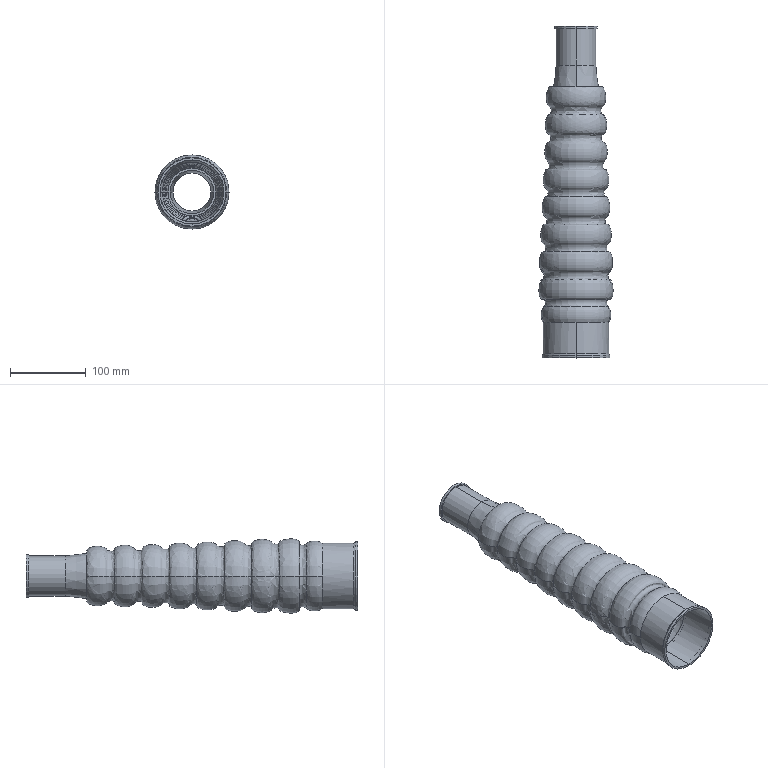Part | STEP file | Electric cylinder dust boot, cylinder A | 1 solid | 60 faces | box 98.284 x 439.582 x 98.284 mm | volume 200790 mm3 | spline 38 | cylinder 12 | plane 6 | cone 4 | commonest cylinder face diameters 50.629 x2 53.029 x2 56.5 x2 85.002 x2 87.402 x2 90.542 x2